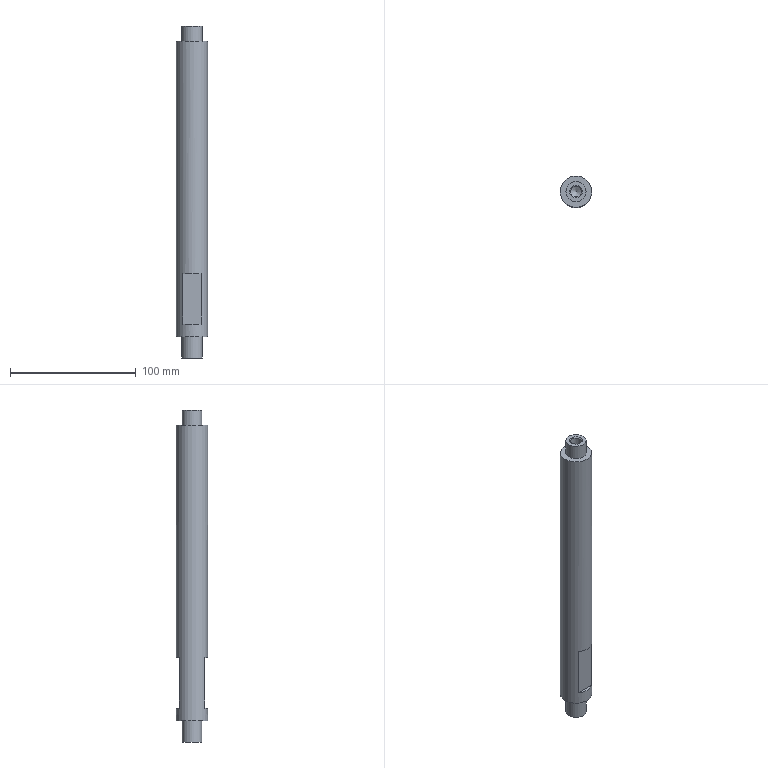Part | STEP file | YBQDJ-QD-PD-2 | 1 solid | 19 faces | box 25 x 25 x 264 mm | volume 116363 mm3 | plane 10 | cylinder 5 | cone 4 | commonest cylinder face diameters 8.5 x2 16 x2 25 x1
STEP:
#1=CARTESIAN_POINT('',(0.,0.,0.));
#2=DIRECTION('',(0.,0.,1.));
#3=DIRECTION('',(1.,0.,0.));
#4=AXIS2_PLACEMENT_3D('',#1,#2,#3);
#5=CARTESIAN_POINT('',(-327.5,-310.,260.));
#6=VERTEX_POINT('',#5);
#7=CARTESIAN_POINT('',(-340.,-310.,260.));
#8=DIRECTION('',(0.,0.,1.));
#9=DIRECTION('',(1.,0.,0.));
#10=AXIS2_PLACEMENT_3D('',#7,#8,#9);
#11=CIRCLE('',#10,12.5);
#12=CARTESIAN_POINT('',(-340.,-310.,270.));
#13=DIRECTION('',(0.,0.,-1.));
#14=DIRECTION('',(-1.,0.,0.));
#15=AXIS2_PLACEMENT_3D('',#12,#13,#14);
#16=CYLINDRICAL_SURFACE('',#15,12.5);
#17=CARTESIAN_POINT('',(9.425,10.));
#18=DIRECTION('',(-1.,0.));
#19=VECTOR('',#18,1.);
#20=LINE('',#17,#19);
#21=(GEOMETRIC_REPRESENTATION_CONTEXT(2)PARAMETRIC_REPRESENTATION_CONTEXT()REPRESENTATION_CONTEXT('',''));
#22=DEFINITIONAL_REPRESENTATION('',(#20),#21);
#23=PCURVE('',#16,#22);
#24=CARTESIAN_POINT('',(-340.,-310.,260.));
#25=DIRECTION('',(0.,0.,1.));
#26=DIRECTION('',(1.,0.,0.));
#27=AXIS2_PLACEMENT_3D('',#24,#25,#26);
#28=PLANE('',#27);
#29=CARTESIAN_POINT('',(0.,0.));
#30=DIRECTION('',(1.,0.));
#31=AXIS2_PLACEMENT_2D('',#29,#30);
#32=CIRCLE('',#31,12.5);
#33=(GEOMETRIC_REPRESENTATION_CONTEXT(2)PARAMETRIC_REPRESENTATION_CONTEXT()REPRESENTATION_CONTEXT('',''));
#34=DEFINITIONAL_REPRESENTATION('',(#32),#33);
#35=PCURVE('',#28,#34);
#36=SURFACE_CURVE('',#11,(#23,#35),.PCURVE_S1.);
#37=EDGE_CURVE('',#6,#6,#36,.T.);
#38=ORIENTED_EDGE('',*,*,#37,.F.);
#39=CARTESIAN_POINT('',(-327.5,-310.,25.));
#40=VERTEX_POINT('',#39);
#41=CARTESIAN_POINT('',(-327.5,-310.,260.));
#42=CARTESIAN_POINT('',(-327.5,-310.,25.));
#43=B_SPLINE_CURVE_WITH_KNOTS('',1,(#41,#42),.UNSPECIFIED.,.F.,.F.,(2,2),(10.,245.),.PIECEWISE_BEZIER_KNOTS.);
#44=CARTESIAN_POINT('',(9.425,0.));
#45=DIRECTION('',(0.,1.));
#46=VECTOR('',#45,1.);
#47=LINE('',#44,#46);
#48=(GEOMETRIC_REPRESENTATION_CONTEXT(2)PARAMETRIC_REPRESENTATION_CONTEXT()REPRESENTATION_CONTEXT('',''));
#49=DEFINITIONAL_REPRESENTATION('',(#47),#48);
#50=PCURVE('',#16,#49);
#51=CARTESIAN_POINT('',(3.142,0.));
#52=DIRECTION('',(0.,1.));
#53=VECTOR('',#52,1.);
#54=LINE('',#51,#53);
#55=(GEOMETRIC_REPRESENTATION_CONTEXT(2)PARAMETRIC_REPRESENTATION_CONTEXT()REPRESENTATION_CONTEXT('',''));
#56=DEFINITIONAL_REPRESENTATION('',(#54),#55);
#57=PCURVE('',#16,#56);
#58=SEAM_CURVE('',#43,(#50,#57),.PCURVE_S1.);
#59=EDGE_CURVE('',#6,#40,#58,.T.);
#60=ORIENTED_EDGE('',*,*,#59,.T.);
#61=CARTESIAN_POINT('',(-340.,-310.,25.));
#62=DIRECTION('',(0.,0.,1.));
#63=DIRECTION('',(1.,0.,0.));
#64=AXIS2_PLACEMENT_3D('',#61,#62,#63);
#65=CIRCLE('',#64,12.5);
#66=CARTESIAN_POINT('',(9.425,245.));
#67=DIRECTION('',(-1.,0.));
#68=VECTOR('',#67,1.);
#69=LINE('',#66,#68);
#70=(GEOMETRIC_REPRESENTATION_CONTEXT(2)PARAMETRIC_REPRESENTATION_CONTEXT()REPRESENTATION_CONTEXT('',''));
#71=DEFINITIONAL_REPRESENTATION('',(#69),#70);
#72=PCURVE('',#16,#71);
#73=CARTESIAN_POINT('',(92.5,10.,25.));
#74=DIRECTION('',(0.,0.,1.));
#75=DIRECTION('',(1.,0.,0.));
#76=AXIS2_PLACEMENT_3D('',#73,#74,#75);
#77=PLANE('',#76);
#78=CARTESIAN_POINT('',(-432.5,-320.));
#79=DIRECTION('',(1.,0.));
#80=AXIS2_PLACEMENT_2D('',#78,#79);
#81=CIRCLE('',#80,12.5);
#82=(GEOMETRIC_REPRESENTATION_CONTEXT(2)PARAMETRIC_REPRESENTATION_CONTEXT()REPRESENTATION_CONTEXT('',''));
#83=DEFINITIONAL_REPRESENTATION('',(#81),#82);
#84=PCURVE('',#77,#83);
#85=SURFACE_CURVE('',#65,(#72,#84),.PCURVE_S1.);
#86=EDGE_CURVE('',#40,#40,#85,.T.);
#87=ORIENTED_EDGE('',*,*,#86,.T.);
#88=ORIENTED_EDGE('',*,*,#59,.F.);
#89=EDGE_LOOP('',(#38,#60,#87,#88));
#90=FACE_BOUND('',#89,.T.);
#91=CARTESIAN_POINT('',(-347.5,-300.,75.));
#92=VERTEX_POINT('',#91);
#93=CARTESIAN_POINT('',(-332.5,-300.,75.));
#94=VERTEX_POINT('',#93);
#95=CARTESIAN_POINT('',(-340.,-310.,75.));
#96=DIRECTION('',(0.,0.,-1.));
#97=DIRECTION('',(0.,1.,0.));
#98=AXIS2_PLACEMENT_3D('',#95,#96,#97);
#99=CIRCLE('',#98,12.5);
#100=CARTESIAN_POINT('',(1.571,195.));
#101=DIRECTION('',(1.,0.));
#102=VECTOR('',#101,1.);
#103=LINE('',#100,#102);
#104=(GEOMETRIC_REPRESENTATION_CONTEXT(2)PARAMETRIC_REPRESENTATION_CONTEXT()REPRESENTATION_CONTEXT('',''));
#105=DEFINITIONAL_REPRESENTATION('',(#103),#104);
#106=PCURVE('',#16,#105);
#107=CARTESIAN_POINT('',(-382.,-300.,75.));
#108=DIRECTION('',(0.,0.,-1.));
#109=DIRECTION('',(0.,1.,0.));
#110=AXIS2_PLACEMENT_3D('',#107,#108,#109);
#111=PLANE('',#110);
#112=CARTESIAN_POINT('',(-10.,42.));
#113=DIRECTION('',(1.,0.));
#114=AXIS2_PLACEMENT_2D('',#112,#113);
#115=CIRCLE('',#114,12.5);
#116=(GEOMETRIC_REPRESENTATION_CONTEXT(2)PARAMETRIC_REPRESENTATION_CONTEXT()REPRESENTATION_CONTEXT('',''));
#117=DEFINITIONAL_REPRESENTATION('',(#115),#116);
#118=PCURVE('',#111,#117);
#119=SURFACE_CURVE('',#99,(#106,#118),.PCURVE_S1.);
#120=EDGE_CURVE('',#92,#94,#119,.T.);
#121=ORIENTED_EDGE('',*,*,#120,.F.);
#122=CARTESIAN_POINT('',(-347.5,-300.,35.));
#123=VERTEX_POINT('',#122);
#124=CARTESIAN_POINT('',(-347.5,-300.,270.));
#125=DIRECTION('',(0.,0.,1.));
#126=VECTOR('',#125,1.);
#127=LINE('',#124,#126);
#128=CARTESIAN_POINT('',(7.21,0.));
#129=DIRECTION('',(0.,-1.));
#130=VECTOR('',#129,1.);
#131=LINE('',#128,#130);
#132=(GEOMETRIC_REPRESENTATION_CONTEXT(2)PARAMETRIC_REPRESENTATION_CONTEXT()REPRESENTATION_CONTEXT('',''));
#133=DEFINITIONAL_REPRESENTATION('',(#131),#132);
#134=PCURVE('',#16,#133);
#135=CARTESIAN_POINT('',(-382.,-300.,35.));
#136=DIRECTION('',(0.,1.,0.));
#137=DIRECTION('',(0.,0.,1.));
#138=AXIS2_PLACEMENT_3D('',#135,#136,#137);
#139=PLANE('',#138);
#140=CARTESIAN_POINT('',(235.,34.5));
#141=DIRECTION('',(1.,0.));
#142=VECTOR('',#141,1.);
#143=LINE('',#140,#142);
#144=(GEOMETRIC_REPRESENTATION_CONTEXT(2)PARAMETRIC_REPRESENTATION_CONTEXT()REPRESENTATION_CONTEXT('',''));
#145=DEFINITIONAL_REPRESENTATION('',(#143),#144);
#146=PCURVE('',#139,#145);
#147=SURFACE_CURVE('',#127,(#134,#146),.PCURVE_S1.);
#148=EDGE_CURVE('',#123,#92,#147,.T.);
#149=ORIENTED_EDGE('',*,*,#148,.F.);
#150=CARTESIAN_POINT('',(-332.5,-300.,35.));
#151=VERTEX_POINT('',#150);
#152=CARTESIAN_POINT('',(-340.,-310.,35.));
#153=DIRECTION('',(0.,0.,1.));
#154=DIRECTION('',(0.,-1.,0.));
#155=AXIS2_PLACEMENT_3D('',#152,#153,#154);
#156=CIRCLE('',#155,12.5);
#157=CARTESIAN_POINT('',(10.996,235.));
#158=DIRECTION('',(-1.,0.));
#159=VECTOR('',#158,1.);
#160=LINE('',#157,#159);
#161=(GEOMETRIC_REPRESENTATION_CONTEXT(2)PARAMETRIC_REPRESENTATION_CONTEXT()REPRESENTATION_CONTEXT('',''));
#162=DEFINITIONAL_REPRESENTATION('',(#160),#161);
#163=PCURVE('',#16,#162);
#164=CARTESIAN_POINT('',(-382.,-281.,35.));
#165=DIRECTION('',(0.,0.,1.));
#166=DIRECTION('',(0.,-1.,0.));
#167=AXIS2_PLACEMENT_3D('',#164,#165,#166);
#168=PLANE('',#167);
#169=CARTESIAN_POINT('',(29.,42.));
#170=DIRECTION('',(1.,0.));
#171=AXIS2_PLACEMENT_2D('',#169,#170);
#172=CIRCLE('',#171,12.5);
#173=(GEOMETRIC_REPRESENTATION_CONTEXT(2)PARAMETRIC_REPRESENTATION_CONTEXT()REPRESENTATION_CONTEXT('',''));
#174=DEFINITIONAL_REPRESENTATION('',(#172),#173);
#175=PCURVE('',#168,#174);
#176=SURFACE_CURVE('',#156,(#163,#175),.PCURVE_S1.);
#177=EDGE_CURVE('',#151,#123,#176,.T.);
#178=ORIENTED_EDGE('',*,*,#177,.F.);
#179=CARTESIAN_POINT('',(-332.5,-300.,270.));
#180=DIRECTION('',(0.,0.,-1.));
#181=VECTOR('',#180,1.);
#182=LINE('',#179,#181);
#183=CARTESIAN_POINT('',(8.497,0.));
#184=DIRECTION('',(0.,1.));
#185=VECTOR('',#184,1.);
#186=LINE('',#183,#185);
#187=(GEOMETRIC_REPRESENTATION_CONTEXT(2)PARAMETRIC_REPRESENTATION_CONTEXT()REPRESENTATION_CONTEXT('',''));
#188=DEFINITIONAL_REPRESENTATION('',(#186),#187);
#189=PCURVE('',#16,#188);
#190=CARTESIAN_POINT('',(235.,49.5));
#191=DIRECTION('',(-1.,0.));
#192=VECTOR('',#191,1.);
#193=LINE('',#190,#192);
#194=(GEOMETRIC_REPRESENTATION_CONTEXT(2)PARAMETRIC_REPRESENTATION_CONTEXT()REPRESENTATION_CONTEXT('',''));
#195=DEFINITIONAL_REPRESENTATION('',(#193),#194);
#196=PCURVE('',#139,#195);
#197=SURFACE_CURVE('',#182,(#189,#196),.PCURVE_S1.);
#198=EDGE_CURVE('',#94,#151,#197,.T.);
#199=ORIENTED_EDGE('',*,*,#198,.F.);
#200=EDGE_LOOP('',(#121,#149,#178,#199));
#201=FACE_BOUND('',#200,.T.);
#202=CARTESIAN_POINT('',(-332.5,-320.,75.));
#203=VERTEX_POINT('',#202);
#204=CARTESIAN_POINT('',(-347.5,-320.,75.));
#205=VERTEX_POINT('',#204);
#206=CARTESIAN_POINT('',(-340.,-310.,75.));
#207=DIRECTION('',(0.,0.,-1.));
#208=DIRECTION('',(0.,1.,0.));
#209=AXIS2_PLACEMENT_3D('',#206,#207,#208);
#210=CIRCLE('',#209,12.5);
#211=CARTESIAN_POINT('',(1.571,195.));
#212=DIRECTION('',(1.,0.));
#213=VECTOR('',#212,1.);
#214=LINE('',#211,#213);
#215=(GEOMETRIC_REPRESENTATION_CONTEXT(2)PARAMETRIC_REPRESENTATION_CONTEXT()REPRESENTATION_CONTEXT('',''));
#216=DEFINITIONAL_REPRESENTATION('',(#214),#215);
#217=PCURVE('',#16,#216);
#218=CARTESIAN_POINT('',(-382.,-339.,75.));
#219=DIRECTION('',(0.,0.,-1.));
#220=DIRECTION('',(0.,1.,0.));
#221=AXIS2_PLACEMENT_3D('',#218,#219,#220);
#222=PLANE('',#221);
#223=CARTESIAN_POINT('',(29.,42.));
#224=DIRECTION('',(1.,0.));
#225=AXIS2_PLACEMENT_2D('',#223,#224);
#226=CIRCLE('',#225,12.5);
#227=(GEOMETRIC_REPRESENTATION_CONTEXT(2)PARAMETRIC_REPRESENTATION_CONTEXT()REPRESENTATION_CONTEXT('',''));
#228=DEFINITIONAL_REPRESENTATION('',(#226),#227);
#229=PCURVE('',#222,#228);
#230=SURFACE_CURVE('',#210,(#217,#229),.PCURVE_S1.);
#231=EDGE_CURVE('',#203,#205,#230,.T.);
#232=ORIENTED_EDGE('',*,*,#231,.F.);
#233=CARTESIAN_POINT('',(-332.5,-320.,35.));
#234=VERTEX_POINT('',#233);
#235=CARTESIAN_POINT('',(-332.5,-320.,270.));
#236=DIRECTION('',(0.,0.,1.));
#237=VECTOR('',#236,1.);
#238=LINE('',#235,#237);
#239=CARTESIAN_POINT('',(4.069,0.));
#240=DIRECTION('',(0.,-1.));
#241=VECTOR('',#240,1.);
#242=LINE('',#239,#241);
#243=(GEOMETRIC_REPRESENTATION_CONTEXT(2)PARAMETRIC_REPRESENTATION_CONTEXT()REPRESENTATION_CONTEXT('',''));
#244=DEFINITIONAL_REPRESENTATION('',(#242),#243);
#245=PCURVE('',#16,#244);
#246=CARTESIAN_POINT('',(-382.,-320.,65.));
#247=DIRECTION('',(0.,-1.,0.));
#248=DIRECTION('',(0.,0.,-1.));
#249=AXIS2_PLACEMENT_3D('',#246,#247,#248);
#250=PLANE('',#249);
#251=CARTESIAN_POINT('',(-205.,49.5));
#252=DIRECTION('',(-1.,0.));
#253=VECTOR('',#252,1.);
#254=LINE('',#251,#253);
#255=(GEOMETRIC_REPRESENTATION_CONTEXT(2)PARAMETRIC_REPRESENTATION_CONTEXT()REPRESENTATION_CONTEXT('',''));
#256=DEFINITIONAL_REPRESENTATION('',(#254),#255);
#257=PCURVE('',#250,#256);
#258=SURFACE_CURVE('',#238,(#245,#257),.PCURVE_S1.);
#259=EDGE_CURVE('',#234,#203,#258,.T.);
#260=ORIENTED_EDGE('',*,*,#259,.F.);
#261=CARTESIAN_POINT('',(-347.5,-320.,35.));
#262=VERTEX_POINT('',#261);
#263=CARTESIAN_POINT('',(-340.,-310.,35.));
#264=DIRECTION('',(0.,0.,1.));
#265=DIRECTION('',(0.,-1.,0.));
#266=AXIS2_PLACEMENT_3D('',#263,#264,#265);
#267=CIRCLE('',#266,12.5);
#268=CARTESIAN_POINT('',(10.996,235.));
#269=DIRECTION('',(-1.,0.));
#270=VECTOR('',#269,1.);
#271=LINE('',#268,#270);
#272=(GEOMETRIC_REPRESENTATION_CONTEXT(2)PARAMETRIC_REPRESENTATION_CONTEXT()REPRESENTATION_CONTEXT('',''));
#273=DEFINITIONAL_REPRESENTATION('',(#271),#272);
#274=PCURVE('',#16,#273);
#275=CARTESIAN_POINT('',(-382.,-320.,35.));
#276=DIRECTION('',(0.,0.,1.));
#277=DIRECTION('',(0.,-1.,0.));
#278=AXIS2_PLACEMENT_3D('',#275,#276,#277);
#279=PLANE('',#278);
#280=CARTESIAN_POINT('',(-10.,42.));
#281=DIRECTION('',(1.,0.));
#282=AXIS2_PLACEMENT_2D('',#280,#281);
#283=CIRCLE('',#282,12.5);
#284=(GEOMETRIC_REPRESENTATION_CONTEXT(2)PARAMETRIC_REPRESENTATION_CONTEXT()REPRESENTATION_CONTEXT('',''));
#285=DEFINITIONAL_REPRESENTATION('',(#283),#284);
#286=PCURVE('',#279,#285);
#287=SURFACE_CURVE('',#267,(#274,#286),.PCURVE_S1.);
#288=EDGE_CURVE('',#262,#234,#287,.T.);
#289=ORIENTED_EDGE('',*,*,#288,.F.);
#290=CARTESIAN_POINT('',(-347.5,-320.,270.));
#291=DIRECTION('',(0.,0.,-1.));
#292=VECTOR('',#291,1.);
#293=LINE('',#290,#292);
#294=CARTESIAN_POINT('',(5.356,0.));
#295=DIRECTION('',(0.,1.));
#296=VECTOR('',#295,1.);
#297=LINE('',#294,#296);
#298=(GEOMETRIC_REPRESENTATION_CONTEXT(2)PARAMETRIC_REPRESENTATION_CONTEXT()REPRESENTATION_CONTEXT('',''));
#299=DEFINITIONAL_REPRESENTATION('',(#297),#298);
#300=PCURVE('',#16,#299);
#301=CARTESIAN_POINT('',(-205.,34.5));
#302=DIRECTION('',(1.,0.));
#303=VECTOR('',#302,1.);
#304=LINE('',#301,#303);
#305=(GEOMETRIC_REPRESENTATION_CONTEXT(2)PARAMETRIC_REPRESENTATION_CONTEXT()REPRESENTATION_CONTEXT('',''));
#306=DEFINITIONAL_REPRESENTATION('',(#304),#305);
#307=PCURVE('',#250,#306);
#308=SURFACE_CURVE('',#293,(#300,#307),.PCURVE_S1.);
#309=EDGE_CURVE('',#205,#262,#308,.T.);
#310=ORIENTED_EDGE('',*,*,#309,.F.);
#311=EDGE_LOOP('',(#232,#260,#289,#310));
#312=FACE_BOUND('',#311,.T.);
#313=ADVANCED_FACE('',(#90,#201,#312),#16,.T.);
#314=CARTESIAN_POINT('',(-332.,-310.,260.));
#315=VERTEX_POINT('',#314);
#316=CARTESIAN_POINT('',(-340.,-310.,260.));
#317=DIRECTION('',(0.,0.,1.));
#318=DIRECTION('',(1.,0.,0.));
#319=AXIS2_PLACEMENT_3D('',#316,#317,#318);
#320=CIRCLE('',#319,8.);
#321=CARTESIAN_POINT('',(0.,0.));
#322=DIRECTION('',(1.,0.));
#323=AXIS2_PLACEMENT_2D('',#321,#322);
#324=CIRCLE('',#323,8.);
#325=(GEOMETRIC_REPRESENTATION_CONTEXT(2)PARAMETRIC_REPRESENTATION_CONTEXT()REPRESENTATION_CONTEXT('',''));
#326=DEFINITIONAL_REPRESENTATION('',(#324),#325);
#327=PCURVE('',#28,#326);
#328=CARTESIAN_POINT('',(-340.,-310.,275.));
#329=DIRECTION('',(0.,0.,-1.));
#330=DIRECTION('',(-1.,0.,0.));
#331=AXIS2_PLACEMENT_3D('',#328,#329,#330);
#332=CYLINDRICAL_SURFACE('',#331,8.);
#333=CARTESIAN_POINT('',(9.425,15.));
#334=DIRECTION('',(-1.,0.));
#335=VECTOR('',#334,1.);
#336=LINE('',#333,#335);
#337=(GEOMETRIC_REPRESENTATION_CONTEXT(2)PARAMETRIC_REPRESENTATION_CONTEXT()REPRESENTATION_CONTEXT('',''));
#338=DEFINITIONAL_REPRESENTATION('',(#336),#337);
#339=PCURVE('',#332,#338);
#340=SURFACE_CURVE('',#320,(#327,#339),.PCURVE_S1.);
#341=EDGE_CURVE('',#315,#315,#340,.T.);
#342=ORIENTED_EDGE('',*,*,#341,.F.);
#343=EDGE_LOOP('',(#342));
#344=FACE_BOUND('',#343,.T.);
#345=ORIENTED_EDGE('',*,*,#37,.T.);
#346=EDGE_LOOP('',(#345));
#347=FACE_BOUND('',#346,.T.);
#348=ADVANCED_FACE('',(#344,#347),#28,.T.);
#349=CARTESIAN_POINT('',(-332.,-310.,25.));
#350=VERTEX_POINT('',#349);
#351=CARTESIAN_POINT('',(-340.,-310.,25.));
#352=DIRECTION('',(0.,0.,-1.));
#353=DIRECTION('',(1.,0.,0.));
#354=AXIS2_PLACEMENT_3D('',#351,#352,#353);
#355=CIRCLE('',#354,8.);
#356=CARTESIAN_POINT('',(-424.5,-320.));
#357=CARTESIAN_POINT('',(-424.5,-333.856));
#358=CARTESIAN_POINT('',(-436.5,-326.928));
#359=CARTESIAN_POINT('',(-448.5,-320.));
#360=CARTESIAN_POINT('',(-436.5,-313.072));
#361=CARTESIAN_POINT('',(-424.5,-306.144));
#362=CARTESIAN_POINT('',(-424.5,-320.));
#363=(BOUNDED_CURVE()B_SPLINE_CURVE(2,(#356,#357,#358,#359,#360,#361,#362),.UNSPECIFIED.,.T.,.F.)B_SPLINE_CURVE_WITH_KNOTS((1,2,2,2,2,1),(-2.094,0.,2.094,4.189,6.283,8.378),.UNSPECIFIED.)CURVE()GEOMETRIC_REPRESENTATION_ITEM()RATIONAL_B_SPLINE_CURVE((1.,0.5,1.,0.5,1.,0.5,1.))REPRESENTATION_ITEM(''));
#364=(GEOMETRIC_REPRESENTATION_CONTEXT(2)PARAMETRIC_REPRESENTATION_CONTEXT()REPRESENTATION_CONTEXT('',''));
#365=DEFINITIONAL_REPRESENTATION('',(#363),#364);
#366=PCURVE('',#77,#365);
#367=CARTESIAN_POINT('',(-340.,-310.,8.));
#368=DIRECTION('',(0.,0.,1.));
#369=DIRECTION('',(1.,0.,0.));
#370=AXIS2_PLACEMENT_3D('',#367,#368,#369);
#371=CYLINDRICAL_SURFACE('',#370,8.);
#372=CARTESIAN_POINT('',(6.283,17.));
#373=DIRECTION('',(-1.,0.));
#374=VECTOR('',#373,1.);
#375=LINE('',#372,#374);
#376=(GEOMETRIC_REPRESENTATION_CONTEXT(2)PARAMETRIC_REPRESENTATION_CONTEXT()REPRESENTATION_CONTEXT('',''));
#377=DEFINITIONAL_REPRESENTATION('',(#375),#376);
#378=PCURVE('',#371,#377);
#379=SURFACE_CURVE('',#355,(#366,#378),.PCURVE_S1.);
#380=EDGE_CURVE('',#350,#350,#379,.T.);
#381=ORIENTED_EDGE('',*,*,#380,.F.);
#382=EDGE_LOOP('',(#381));
#383=FACE_BOUND('',#382,.T.);
#384=ORIENTED_EDGE('',*,*,#86,.F.);
#385=EDGE_LOOP('',(#384));
#386=FACE_BOUND('',#385,.T.);
#387=ADVANCED_FACE('',(#383,#386),#77,.F.);
#388=CARTESIAN_POINT('',(-332.,-310.,272.));
#389=VERTEX_POINT('',#388);
#390=CARTESIAN_POINT('',(-340.,-310.,272.));
#391=DIRECTION('',(0.,0.,1.));
#392=DIRECTION('',(1.,0.,0.));
#393=AXIS2_PLACEMENT_3D('',#390,#391,#392);
#394=CIRCLE('',#393,8.);
#395=CARTESIAN_POINT('',(9.425,3.));
#396=DIRECTION('',(-1.,0.));
#397=VECTOR('',#396,1.);
#398=LINE('',#395,#397);
#399=(GEOMETRIC_REPRESENTATION_CONTEXT(2)PARAMETRIC_REPRESENTATION_CONTEXT()REPRESENTATION_CONTEXT('',''));
#400=DEFINITIONAL_REPRESENTATION('',(#398),#399);
#401=PCURVE('',#332,#400);
#402=CARTESIAN_POINT('',(-340.,-310.,272.));
#403=DIRECTION('',(0.,0.,1.));
#404=DIRECTION('',(1.,0.,0.));
#405=AXIS2_PLACEMENT_3D('',#402,#403,#404);
#406=PLANE('',#405);
#407=CARTESIAN_POINT('',(0.,0.));
#408=DIRECTION('',(1.,0.));
#409=AXIS2_PLACEMENT_2D('',#407,#408);
#410=CIRCLE('',#409,8.);
#411=(GEOMETRIC_REPRESENTATION_CONTEXT(2)PARAMETRIC_REPRESENTATION_CONTEXT()REPRESENTATION_CONTEXT('',''));
#412=DEFINITIONAL_REPRESENTATION('',(#410),#411);
#413=PCURVE('',#406,#412);
#414=SURFACE_CURVE('',#394,(#401,#413),.PCURVE_S1.);
#415=EDGE_CURVE('',#389,#389,#414,.T.);
#416=ORIENTED_EDGE('',*,*,#415,.F.);
#417=CARTESIAN_POINT('',(-332.,-310.,272.));
#418=CARTESIAN_POINT('',(-332.,-310.,260.));
#419=B_SPLINE_CURVE_WITH_KNOTS('',1,(#417,#418),.UNSPECIFIED.,.F.,.F.,(2,2),(3.,15.),.PIECEWISE_BEZIER_KNOTS.);
#420=CARTESIAN_POINT('',(9.425,0.));
#421=DIRECTION('',(0.,1.));
#422=VECTOR('',#421,1.);
#423=LINE('',#420,#422);
#424=(GEOMETRIC_REPRESENTATION_CONTEXT(2)PARAMETRIC_REPRESENTATION_CONTEXT()REPRESENTATION_CONTEXT('',''));
#425=DEFINITIONAL_REPRESENTATION('',(#423),#424);
#426=PCURVE('',#332,#425);
#427=CARTESIAN_POINT('',(3.142,0.));
#428=DIRECTION('',(0.,1.));
#429=VECTOR('',#428,1.);
#430=LINE('',#427,#429);
#431=(GEOMETRIC_REPRESENTATION_CONTEXT(2)PARAMETRIC_REPRESENTATION_CONTEXT()REPRESENTATION_CONTEXT('',''));
#432=DEFINITIONAL_REPRESENTATION('',(#430),#431);
#433=PCURVE('',#332,#432);
#434=SEAM_CURVE('',#419,(#426,#433),.PCURVE_S1.);
#435=EDGE_CURVE('',#389,#315,#434,.T.);
#436=ORIENTED_EDGE('',*,*,#435,.T.);
#437=ORIENTED_EDGE('',*,*,#341,.T.);
#438=ORIENTED_EDGE('',*,*,#435,.F.);
#439=EDGE_LOOP('',(#416,#436,#437,#438));
#440=FACE_BOUND('',#439,.T.);
#441=ADVANCED_FACE('',(#440),#332,.T.);
#442=CARTESIAN_POINT('',(-335.,-310.,272.));
#443=VERTEX_POINT('',#442);
#444=CARTESIAN_POINT('',(-340.,-310.,272.));
#445=DIRECTION('',(0.,0.,-1.));
#446=DIRECTION('',(1.,0.,0.));
#447=AXIS2_PLACEMENT_3D('',#444,#445,#446);
#448=CIRCLE('',#447,5.);
#449=CARTESIAN_POINT('',(5.,0.));
#450=CARTESIAN_POINT('',(5.,-8.66));
#451=CARTESIAN_POINT('',(-2.5,-4.33));
#452=CARTESIAN_POINT('',(-10.,0.));
#453=CARTESIAN_POINT('',(-2.5,4.33));
#454=CARTESIAN_POINT('',(5.,8.66));
#455=CARTESIAN_POINT('',(5.,0.));
#456=(BOUNDED_CURVE()B_SPLINE_CURVE(2,(#449,#450,#451,#452,#453,#454,#455),.UNSPECIFIED.,.T.,.F.)B_SPLINE_CURVE_WITH_KNOTS((1,2,2,2,2,1),(-2.094,0.,2.094,4.189,6.283,8.378),.UNSPECIFIED.)CURVE()GEOMETRIC_REPRESENTATION_ITEM()RATIONAL_B_SPLINE_CURVE((1.,0.5,1.,0.5,1.,0.5,1.))REPRESENTATION_ITEM(''));
#457=(GEOMETRIC_REPRESENTATION_CONTEXT(2)PARAMETRIC_REPRESENTATION_CONTEXT()REPRESENTATION_CONTEXT('',''));
#458=DEFINITIONAL_REPRESENTATION('',(#456),#457);
#459=PCURVE('',#406,#458);
#460=CARTESIAN_POINT('',(-340.,-310.,272.));
#461=DIRECTION('',(0.,0.,1.));
#462=DIRECTION('',(1.,0.,0.));
#463=AXIS2_PLACEMENT_3D('',#460,#461,#462);
#464=CONICAL_SURFACE('',#463,5.,0.7854);
#465=CARTESIAN_POINT('',(6.283,0.));
#466=DIRECTION('',(-1.,0.));
#467=VECTOR('',#466,1.);
#468=LINE('',#465,#467);
#469=(GEOMETRIC_REPRESENTATION_CONTEXT(2)PARAMETRIC_REPRESENTATION_CONTEXT()REPRESENTATION_CONTEXT('',''));
#470=DEFINITIONAL_REPRESENTATION('',(#468),#469);
#471=PCURVE('',#464,#470);
#472=SURFACE_CURVE('',#448,(#459,#471),.PCURVE_S1.);
#473=EDGE_CURVE('',#443,#443,#472,.T.);
#474=ORIENTED_EDGE('',*,*,#473,.T.);
#475=EDGE_LOOP('',(#474));
#476=FACE_BOUND('',#475,.T.);
#477=ORIENTED_EDGE('',*,*,#415,.T.);
#478=EDGE_LOOP('',(#477));
#479=FACE_BOUND('',#478,.T.);
#480=ADVANCED_FACE('',(#476,#479),#406,.T.);
#481=CARTESIAN_POINT('',(-335.75,-310.,250.));
#482=VERTEX_POINT('',#481);
#483=CARTESIAN_POINT('',(-344.25,-310.,250.));
#484=VERTEX_POINT('',#483);
#485=CARTESIAN_POINT('',(-340.,-310.,250.));
#486=DIRECTION('',(0.,0.,1.));
#487=DIRECTION('',(-1.,0.,0.));
#488=AXIS2_PLACEMENT_3D('',#485,#486,#487);
#489=CIRCLE('',#488,4.25);
#490=CARTESIAN_POINT('',(-340.,-310.,250.));
#491=DIRECTION('',(0.,0.,1.));
#492=DIRECTION('',(1.,0.,0.));
#493=AXIS2_PLACEMENT_3D('',#490,#491,#492);
#494=CONICAL_SURFACE('',#493,4.25,1.03);
#495=CARTESIAN_POINT('',(-3.142,0.));
#496=DIRECTION('',(1.,0.));
#497=VECTOR('',#496,1.);
#498=LINE('',#495,#497);
#499=(GEOMETRIC_REPRESENTATION_CONTEXT(2)PARAMETRIC_REPRESENTATION_CONTEXT()REPRESENTATION_CONTEXT('',''));
#500=DEFINITIONAL_REPRESENTATION('',(#498),#499);
#501=PCURVE('',#494,#500);
#502=CARTESIAN_POINT('',(-340.,-310.,275.));
#503=DIRECTION('',(0.,0.,-1.));
#504=DIRECTION('',(-1.,0.,0.));
#505=AXIS2_PLACEMENT_3D('',#502,#503,#504);
#506=CYLINDRICAL_SURFACE('',#505,4.25);
#507=CARTESIAN_POINT('',(12.566,25.));
#508=DIRECTION('',(-1.,0.));
#509=VECTOR('',#508,1.);
#510=LINE('',#507,#509);
#511=(GEOMETRIC_REPRESENTATION_CONTEXT(2)PARAMETRIC_REPRESENTATION_CONTEXT()REPRESENTATION_CONTEXT('',''));
#512=DEFINITIONAL_REPRESENTATION('',(#510),#511);
#513=PCURVE('',#506,#512);
#514=SURFACE_CURVE('',#489,(#501,#513),.PCURVE_S1.);
#515=EDGE_CURVE('',#482,#484,#514,.T.);
#516=ORIENTED_EDGE('',*,*,#515,.F.);
#517=CARTESIAN_POINT('',(-340.,-310.,247.446));
#518=VERTEX_POINT('',#517);
#519=CARTESIAN_POINT('',(-340.,-310.,247.446));
#520=CARTESIAN_POINT('',(-335.75,-310.,250.));
#521=B_SPLINE_CURVE_WITH_KNOTS('',1,(#519,#520),.UNSPECIFIED.,.F.,.F.,(2,2),(-4.958,0.),.PIECEWISE_BEZIER_KNOTS.);
#522=CARTESIAN_POINT('',(0.,0.));
#523=DIRECTION('',(0.,1.));
#524=VECTOR('',#523,1.);
#525=LINE('',#522,#524);
#526=(GEOMETRIC_REPRESENTATION_CONTEXT(2)PARAMETRIC_REPRESENTATION_CONTEXT()REPRESENTATION_CONTEXT('',''));
#527=DEFINITIONAL_REPRESENTATION('',(#525),#526);
#528=PCURVE('',#494,#527);
#529=CARTESIAN_POINT('',(6.283,0.));
#530=DIRECTION('',(0.,1.));
#531=VECTOR('',#530,1.);
#532=LINE('',#529,#531);
#533=(GEOMETRIC_REPRESENTATION_CONTEXT(2)PARAMETRIC_REPRESENTATION_CONTEXT()REPRESENTATION_CONTEXT('',''));
#534=DEFINITIONAL_REPRESENTATION('',(#532),#533);
#535=PCURVE('',#494,#534);
#536=SEAM_CURVE('',#521,(#528,#535),.PCURVE_S1.);
#537=EDGE_CURVE('',#518,#482,#536,.T.);
#538=ORIENTED_EDGE('',*,*,#537,.F.);
#539=ORIENTED_EDGE('',*,*,#537,.T.);
#540=CARTESIAN_POINT('',(-340.,-310.,250.));
#541=DIRECTION('',(0.,0.,1.));
#542=DIRECTION('',(-1.,0.,0.));
#543=AXIS2_PLACEMENT_3D('',#540,#541,#542);
#544=CIRCLE('',#543,4.25);
#545=CARTESIAN_POINT('',(3.142,0.));
#546=DIRECTION('',(1.,0.));
#547=VECTOR('',#546,1.);
#548=LINE('',#545,#547);
#549=(GEOMETRIC_REPRESENTATION_CONTEXT(2)PARAMETRIC_REPRESENTATION_CONTEXT()REPRESENTATION_CONTEXT('',''));
#550=DEFINITIONAL_REPRESENTATION('',(#548),#549);
#551=PCURVE('',#494,#550);
#552=CARTESIAN_POINT('',(6.283,25.));
#553=DIRECTION('',(-1.,0.));
#554=VECTOR('',#553,1.);
#555=LINE('',#552,#554);
#556=(GEOMETRIC_REPRESENTATION_CONTEXT(2)PARAMETRIC_REPRESENTATION_CONTEXT()REPRESENTATION_CONTEXT('',''));
#557=DEFINITIONAL_REPRESENTATION('',(#555),#556);
#558=PCURVE('',#506,#557);
#559=SURFACE_CURVE('',#544,(#551,#558),.PCURVE_S1.);
#560=EDGE_CURVE('',#484,#482,#559,.T.);
#561=ORIENTED_EDGE('',*,*,#560,.F.);
#562=EDGE_LOOP('',(#516,#538,#539,#561));
#563=FACE_BOUND('',#562,.F.);
#564=ADVANCED_FACE('',(#563),#494,.F.);
#565=CARTESIAN_POINT('',(-335.75,-310.,271.25));
#566=VERTEX_POINT('',#565);
#567=CARTESIAN_POINT('',(-340.,-310.,271.25));
#568=DIRECTION('',(0.,0.,1.));
#569=DIRECTION('',(1.,0.,0.));
#570=AXIS2_PLACEMENT_3D('',#567,#568,#569);
#571=CIRCLE('',#570,4.25);
#572=CARTESIAN_POINT('',(9.425,3.75));
#573=DIRECTION('',(-1.,0.));
#574=VECTOR('',#573,1.);
#575=LINE('',#572,#574);
#576=(GEOMETRIC_REPRESENTATION_CONTEXT(2)PARAMETRIC_REPRESENTATION_CONTEXT()REPRESENTATION_CONTEXT('',''));
#577=DEFINITIONAL_REPRESENTATION('',(#575),#576);
#578=PCURVE('',#506,#577);
#579=CARTESIAN_POINT('',(0.,-0.75));
#580=DIRECTION('',(1.,0.));
#581=VECTOR('',#580,1.);
#582=LINE('',#579,#581);
#583=(GEOMETRIC_REPRESENTATION_CONTEXT(2)PARAMETRIC_REPRESENTATION_CONTEXT()REPRESENTATION_CONTEXT('',''));
#584=DEFINITIONAL_REPRESENTATION('',(#582),#583);
#585=PCURVE('',#464,#584);
#586=SURFACE_CURVE('',#571,(#578,#585),.PCURVE_S1.);
#587=EDGE_CURVE('',#566,#566,#586,.T.);
#588=ORIENTED_EDGE('',*,*,#587,.F.);
#589=CARTESIAN_POINT('',(-335.75,-310.,271.25));
#590=CARTESIAN_POINT('',(-335.75,-310.,250.));
#591=B_SPLINE_CURVE_WITH_KNOTS('',1,(#589,#590),.UNSPECIFIED.,.F.,.F.,(2,2),(3.75,25.),.PIECEWISE_BEZIER_KNOTS.);
#592=CARTESIAN_POINT('',(9.425,0.));
#593=DIRECTION('',(0.,1.));
#594=VECTOR('',#593,1.);
#595=LINE('',#592,#594);
#596=(GEOMETRIC_REPRESENTATION_CONTEXT(2)PARAMETRIC_REPRESENTATION_CONTEXT()REPRESENTATION_CONTEXT('',''));
#597=DEFINITIONAL_REPRESENTATION('',(#595),#596);
#598=PCURVE('',#506,#597);
#599=CARTESIAN_POINT('',(3.142,0.));
#600=DIRECTION('',(0.,1.));
#601=VECTOR('',#600,1.);
#602=LINE('',#599,#601);
#603=(GEOMETRIC_REPRESENTATION_CONTEXT(2)PARAMETRIC_REPRESENTATION_CONTEXT()REPRESENTATION_CONTEXT('',''));
#604=DEFINITIONAL_REPRESENTATION('',(#602),#603);
#605=PCURVE('',#506,#604);
#606=SEAM_CURVE('',#591,(#598,#605),.PCURVE_S1.);
#607=EDGE_CURVE('',#566,#482,#606,.T.);
#608=ORIENTED_EDGE('',*,*,#607,.T.);
#609=ORIENTED_EDGE('',*,*,#515,.T.);
#610=ORIENTED_EDGE('',*,*,#560,.T.);
#611=ORIENTED_EDGE('',*,*,#607,.F.);
#612=EDGE_LOOP('',(#588,#608,#609,#610,#611));
#613=FACE_BOUND('',#612,.F.);
#614=ADVANCED_FACE('',(#613),#506,.F.);
#615=ORIENTED_EDGE('',*,*,#587,.T.);
#616=CARTESIAN_POINT('',(-335.75,-310.,271.25));
#617=CARTESIAN_POINT('',(-335.,-310.,272.));
#618=B_SPLINE_CURVE_WITH_KNOTS('',1,(#616,#617),.UNSPECIFIED.,.F.,.F.,(2,2),(-1.061,0.),.PIECEWISE_BEZIER_KNOTS.);
#619=CARTESIAN_POINT('',(6.283,0.));
#620=DIRECTION('',(0.,1.));
#621=VECTOR('',#620,1.);
#622=LINE('',#619,#621);
#623=(GEOMETRIC_REPRESENTATION_CONTEXT(2)PARAMETRIC_REPRESENTATION_CONTEXT()REPRESENTATION_CONTEXT('',''));
#624=DEFINITIONAL_REPRESENTATION('',(#622),#623);
#625=PCURVE('',#464,#624);
#626=CARTESIAN_POINT('',(0.,0.));
#627=DIRECTION('',(0.,1.));
#628=VECTOR('',#627,1.);
#629=LINE('',#626,#628);
#630=(GEOMETRIC_REPRESENTATION_CONTEXT(2)PARAMETRIC_REPRESENTATION_CONTEXT()REPRESENTATION_CONTEXT('',''));
#631=DEFINITIONAL_REPRESENTATION('',(#629),#630);
#632=PCURVE('',#464,#631);
#633=SEAM_CURVE('',#618,(#625,#632),.PCURVE_S1.);
#634=EDGE_CURVE('',#566,#443,#633,.T.);
#635=ORIENTED_EDGE('',*,*,#634,.T.);
#636=ORIENTED_EDGE('',*,*,#473,.T.);
#637=ORIENTED_EDGE('',*,*,#634,.F.);
#638=EDGE_LOOP('',(#615,#635,#636,#637));
#639=FACE_BOUND('',#638,.F.);
#640=ADVANCED_FACE('',(#639),#464,.F.);
#641=CARTESIAN_POINT('',(-332.,-310.,8.));
#642=VERTEX_POINT('',#641);
#643=CARTESIAN_POINT('',(-348.,-310.,8.));
#644=VERTEX_POINT('',#643);
#645=CARTESIAN_POINT('',(-340.,-310.,8.));
#646=DIRECTION('',(0.,0.,-1.));
#647=DIRECTION('',(-1.,0.,0.));
#648=AXIS2_PLACEMENT_3D('',#645,#646,#647);
#649=CIRCLE('',#648,8.);
#650=CARTESIAN_POINT('',(9.425,0.));
#651=DIRECTION('',(-1.,0.));
#652=VECTOR('',#651,1.);
#653=LINE('',#650,#652);
#654=(GEOMETRIC_REPRESENTATION_CONTEXT(2)PARAMETRIC_REPRESENTATION_CONTEXT()REPRESENTATION_CONTEXT('',''));
#655=DEFINITIONAL_REPRESENTATION('',(#653),#654);
#656=PCURVE('',#371,#655);
#657=CARTESIAN_POINT('',(-340.,-310.,8.));
#658=DIRECTION('',(0.,0.,-1.));
#659=DIRECTION('',(-1.,0.,0.));
#660=AXIS2_PLACEMENT_3D('',#657,#658,#659);
#661=PLANE('',#660);
#662=CARTESIAN_POINT('',(0.,0.));
#663=DIRECTION('',(1.,0.));
#664=AXIS2_PLACEMENT_2D('',#662,#663);
#665=CIRCLE('',#664,8.);
#666=(GEOMETRIC_REPRESENTATION_CONTEXT(2)PARAMETRIC_REPRESENTATION_CONTEXT()REPRESENTATION_CONTEXT('',''));
#667=DEFINITIONAL_REPRESENTATION('',(#665),#666);
#668=PCURVE('',#661,#667);
#669=SURFACE_CURVE('',#649,(#656,#668),.PCURVE_S1.);
#670=EDGE_CURVE('',#642,#644,#669,.T.);
#671=ORIENTED_EDGE('',*,*,#670,.F.);
#672=CARTESIAN_POINT('',(-332.,-310.,8.));
#673=CARTESIAN_POINT('',(-332.,-310.,25.));
#674=B_SPLINE_CURVE_WITH_KNOTS('',1,(#672,#673),.UNSPECIFIED.,.F.,.F.,(2,2),(0.,17.),.PIECEWISE_BEZIER_KNOTS.);
#675=CARTESIAN_POINT('',(6.283,0.));
#676=DIRECTION('',(0.,1.));
#677=VECTOR('',#676,1.);
#678=LINE('',#675,#677);
#679=(GEOMETRIC_REPRESENTATION_CONTEXT(2)PARAMETRIC_REPRESENTATION_CONTEXT()REPRESENTATION_CONTEXT('',''));
#680=DEFINITIONAL_REPRESENTATION('',(#678),#679);
#681=PCURVE('',#371,#680);
#682=CARTESIAN_POINT('',(0.,0.));
#683=DIRECTION('',(0.,1.));
#684=VECTOR('',#683,1.);
#685=LINE('',#682,#684);
#686=(GEOMETRIC_REPRESENTATION_CONTEXT(2)PARAMETRIC_REPRESENTATION_CONTEXT()REPRESENTATION_CONTEXT('',''));
#687=DEFINITIONAL_REPRESENTATION('',(#685),#686);
#688=PCURVE('',#371,#687);
#689=SEAM_CURVE('',#674,(#681,#688),.PCURVE_S1.);
#690=EDGE_CURVE('',#642,#350,#689,.T.);
#691=ORIENTED_EDGE('',*,*,#690,.T.);
#692=ORIENTED_EDGE('',*,*,#380,.T.);
#693=ORIENTED_EDGE('',*,*,#690,.F.);
#694=CARTESIAN_POINT('',(-340.,-310.,8.));
#695=DIRECTION('',(0.,0.,-1.));
#696=DIRECTION('',(-1.,0.,0.));
#697=AXIS2_PLACEMENT_3D('',#694,#695,#696);
#698=CIRCLE('',#697,8.);
#699=CARTESIAN_POINT('',(3.142,0.));
#700=DIRECTION('',(-1.,0.));
#701=VECTOR('',#700,1.);
#702=LINE('',#699,#701);
#703=(GEOMETRIC_REPRESENTATION_CONTEXT(2)PARAMETRIC_REPRESENTATION_CONTEXT()REPRESENTATION_CONTEXT('',''));
#704=DEFINITIONAL_REPRESENTATION('',(#702),#703);
#705=PCURVE('',#371,#704);
#706=CARTESIAN_POINT('',(0.,0.));
#707=DIRECTION('',(1.,0.));
#708=AXIS2_PLACEMENT_2D('',#706,#707);
#709=CIRCLE('',#708,8.);
#710=(GEOMETRIC_REPRESENTATION_CONTEXT(2)PARAMETRIC_REPRESENTATION_CONTEXT()REPRESENTATION_CONTEXT('',''));
#711=DEFINITIONAL_REPRESENTATION('',(#709),#710);
#712=PCURVE('',#661,#711);
#713=SURFACE_CURVE('',#698,(#705,#712),.PCURVE_S1.);
#714=EDGE_CURVE('',#644,#642,#713,.T.);
#715=ORIENTED_EDGE('',*,*,#714,.F.);
#716=EDGE_LOOP('',(#671,#691,#692,#693,#715));
#717=FACE_BOUND('',#716,.T.);
#718=ADVANCED_FACE('',(#717),#371,.T.);
#719=CARTESIAN_POINT('',(-345.,-310.,8.));
#720=VERTEX_POINT('',#719);
#721=CARTESIAN_POINT('',(-340.,-310.,8.));
#722=DIRECTION('',(0.,0.,1.));
#723=DIRECTION('',(-1.,0.,0.));
#724=AXIS2_PLACEMENT_3D('',#721,#722,#723);
#725=CIRCLE('',#724,5.);
#726=CARTESIAN_POINT('',(5.,0.));
#727=CARTESIAN_POINT('',(5.,-8.66));
#728=CARTESIAN_POINT('',(-2.5,-4.33));
#729=CARTESIAN_POINT('',(-10.,0.));
#730=CARTESIAN_POINT('',(-2.5,4.33));
#731=CARTESIAN_POINT('',(5.,8.66));
#732=CARTESIAN_POINT('',(5.,0.));
#733=(BOUNDED_CURVE()B_SPLINE_CURVE(2,(#726,#727,#728,#729,#730,#731,#732),.UNSPECIFIED.,.T.,.F.)B_SPLINE_CURVE_WITH_KNOTS((1,2,2,2,2,1),(-2.094,0.,2.094,4.189,6.283,8.378),.UNSPECIFIED.)CURVE()GEOMETRIC_REPRESENTATION_ITEM()RATIONAL_B_SPLINE_CURVE((1.,0.5,1.,0.5,1.,0.5,1.))REPRESENTATION_ITEM(''));
#734=(GEOMETRIC_REPRESENTATION_CONTEXT(2)PARAMETRIC_REPRESENTATION_CONTEXT()REPRESENTATION_CONTEXT('',''));
#735=DEFINITIONAL_REPRESENTATION('',(#733),#734);
#736=PCURVE('',#661,#735);
#737=CARTESIAN_POINT('',(-340.,-310.,8.));
#738=DIRECTION('',(0.,0.,-1.));
#739=DIRECTION('',(-1.,0.,0.));
#740=AXIS2_PLACEMENT_3D('',#737,#738,#739);
#741=CONICAL_SURFACE('',#740,5.,0.7854);
#742=CARTESIAN_POINT('',(6.283,0.));
#743=DIRECTION('',(-1.,0.));
#744=VECTOR('',#743,1.);
#745=LINE('',#742,#744);
#746=(GEOMETRIC_REPRESENTATION_CONTEXT(2)PARAMETRIC_REPRESENTATION_CONTEXT()REPRESENTATION_CONTEXT('',''));
#747=DEFINITIONAL_REPRESENTATION('',(#745),#746);
#748=PCURVE('',#741,#747);
#749=SURFACE_CURVE('',#725,(#736,#748),.PCURVE_S1.);
#750=EDGE_CURVE('',#720,#720,#749,.T.);
#751=ORIENTED_EDGE('',*,*,#750,.T.);
#752=EDGE_LOOP('',(#751));
#753=FACE_BOUND('',#752,.T.);
#754=ORIENTED_EDGE('',*,*,#714,.T.);
#755=ORIENTED_EDGE('',*,*,#670,.T.);
#756=EDGE_LOOP('',(#754,#755));
#757=FACE_BOUND('',#756,.T.);
#758=ADVANCED_FACE('',(#753,#757),#661,.T.);
#759=CARTESIAN_POINT('',(-344.25,-310.,33.));
#760=VERTEX_POINT('',#759);
#761=CARTESIAN_POINT('',(-335.75,-310.,33.));
#762=VERTEX_POINT('',#761);
#763=CARTESIAN_POINT('',(-340.,-310.,33.));
#764=DIRECTION('',(0.,0.,-1.));
#765=DIRECTION('',(1.,0.,0.));
#766=AXIS2_PLACEMENT_3D('',#763,#764,#765);
#767=CIRCLE('',#766,4.25);
#768=CARTESIAN_POINT('',(-340.,-310.,33.));
#769=DIRECTION('',(0.,0.,-1.));
#770=DIRECTION('',(-1.,0.,0.));
#771=AXIS2_PLACEMENT_3D('',#768,#769,#770);
#772=CONICAL_SURFACE('',#771,4.25,1.03);
#773=CARTESIAN_POINT('',(-3.142,0.));
#774=DIRECTION('',(1.,0.));
#775=VECTOR('',#774,1.);
#776=LINE('',#773,#775);
#777=(GEOMETRIC_REPRESENTATION_CONTEXT(2)PARAMETRIC_REPRESENTATION_CONTEXT()REPRESENTATION_CONTEXT('',''));
#778=DEFINITIONAL_REPRESENTATION('',(#776),#777);
#779=PCURVE('',#772,#778);
#780=CARTESIAN_POINT('',(-340.,-310.,8.));
#781=DIRECTION('',(0.,0.,1.));
#782=DIRECTION('',(1.,0.,0.));
#783=AXIS2_PLACEMENT_3D('',#780,#781,#782);
#784=CYLINDRICAL_SURFACE('',#783,4.25);
#785=CARTESIAN_POINT('',(12.566,25.));
#786=DIRECTION('',(-1.,0.));
#787=VECTOR('',#786,1.);
#788=LINE('',#785,#787);
#789=(GEOMETRIC_REPRESENTATION_CONTEXT(2)PARAMETRIC_REPRESENTATION_CONTEXT()REPRESENTATION_CONTEXT('',''));
#790=DEFINITIONAL_REPRESENTATION('',(#788),#789);
#791=PCURVE('',#784,#790);
#792=SURFACE_CURVE('',#767,(#779,#791),.PCURVE_S1.);
#793=EDGE_CURVE('',#760,#762,#792,.T.);
#794=ORIENTED_EDGE('',*,*,#793,.F.);
#795=CARTESIAN_POINT('',(-340.,-310.,35.554));
#796=VERTEX_POINT('',#795);
#797=CARTESIAN_POINT('',(-340.,-310.,35.554));
#798=CARTESIAN_POINT('',(-344.25,-310.,33.));
#799=B_SPLINE_CURVE_WITH_KNOTS('',1,(#797,#798),.UNSPECIFIED.,.F.,.F.,(2,2),(-4.958,0.),.PIECEWISE_BEZIER_KNOTS.);
#800=CARTESIAN_POINT('',(0.,0.));
#801=DIRECTION('',(0.,1.));
#802=VECTOR('',#801,1.);
#803=LINE('',#800,#802);
#804=(GEOMETRIC_REPRESENTATION_CONTEXT(2)PARAMETRIC_REPRESENTATION_CONTEXT()REPRESENTATION_CONTEXT('',''));
#805=DEFINITIONAL_REPRESENTATION('',(#803),#804);
#806=PCURVE('',#772,#805);
#807=CARTESIAN_POINT('',(6.283,0.));
#808=DIRECTION('',(0.,1.));
#809=VECTOR('',#808,1.);
#810=LINE('',#807,#809);
#811=(GEOMETRIC_REPRESENTATION_CONTEXT(2)PARAMETRIC_REPRESENTATION_CONTEXT()REPRESENTATION_CONTEXT('',''));
#812=DEFINITIONAL_REPRESENTATION('',(#810),#811);
#813=PCURVE('',#772,#812);
#814=SEAM_CURVE('',#799,(#806,#813),.PCURVE_S1.);
#815=EDGE_CURVE('',#796,#760,#814,.T.);
#816=ORIENTED_EDGE('',*,*,#815,.F.);
#817=ORIENTED_EDGE('',*,*,#815,.T.);
#818=CARTESIAN_POINT('',(-340.,-310.,33.));
#819=DIRECTION('',(0.,0.,-1.));
#820=DIRECTION('',(1.,0.,0.));
#821=AXIS2_PLACEMENT_3D('',#818,#819,#820);
#822=CIRCLE('',#821,4.25);
#823=CARTESIAN_POINT('',(3.142,0.));
#824=DIRECTION('',(1.,0.));
#825=VECTOR('',#824,1.);
#826=LINE('',#823,#825);
#827=(GEOMETRIC_REPRESENTATION_CONTEXT(2)PARAMETRIC_REPRESENTATION_CONTEXT()REPRESENTATION_CONTEXT('',''));
#828=DEFINITIONAL_REPRESENTATION('',(#826),#827);
#829=PCURVE('',#772,#828);
#830=CARTESIAN_POINT('',(6.283,25.));
#831=DIRECTION('',(-1.,0.));
#832=VECTOR('',#831,1.);
#833=LINE('',#830,#832);
#834=(GEOMETRIC_REPRESENTATION_CONTEXT(2)PARAMETRIC_REPRESENTATION_CONTEXT()REPRESENTATION_CONTEXT('',''));
#835=DEFINITIONAL_REPRESENTATION('',(#833),#834);
#836=PCURVE('',#784,#835);
#837=SURFACE_CURVE('',#822,(#829,#836),.PCURVE_S1.);
#838=EDGE_CURVE('',#762,#760,#837,.T.);
#839=ORIENTED_EDGE('',*,*,#838,.F.);
#840=EDGE_LOOP('',(#794,#816,#817,#839));
#841=FACE_BOUND('',#840,.F.);
#842=ADVANCED_FACE('',(#841),#772,.F.);
#843=CARTESIAN_POINT('',(-344.25,-310.,8.75));
#844=VERTEX_POINT('',#843);
#845=CARTESIAN_POINT('',(-340.,-310.,8.75));
#846=DIRECTION('',(0.,0.,-1.));
#847=DIRECTION('',(-1.,0.,0.));
#848=AXIS2_PLACEMENT_3D('',#845,#846,#847);
#849=CIRCLE('',#848,4.25);
#850=CARTESIAN_POINT('',(9.425,0.75));
#851=DIRECTION('',(-1.,0.));
#852=VECTOR('',#851,1.);
#853=LINE('',#850,#852);
#854=(GEOMETRIC_REPRESENTATION_CONTEXT(2)PARAMETRIC_REPRESENTATION_CONTEXT()REPRESENTATION_CONTEXT('',''));
#855=DEFINITIONAL_REPRESENTATION('',(#853),#854);
#856=PCURVE('',#784,#855);
#857=CARTESIAN_POINT('',(0.,-0.75));
#858=DIRECTION('',(1.,0.));
#859=VECTOR('',#858,1.);
#860=LINE('',#857,#859);
#861=(GEOMETRIC_REPRESENTATION_CONTEXT(2)PARAMETRIC_REPRESENTATION_CONTEXT()REPRESENTATION_CONTEXT('',''));
#862=DEFINITIONAL_REPRESENTATION('',(#860),#861);
#863=PCURVE('',#741,#862);
#864=SURFACE_CURVE('',#849,(#856,#863),.PCURVE_S1.);
#865=EDGE_CURVE('',#844,#844,#864,.T.);
#866=ORIENTED_EDGE('',*,*,#865,.F.);
#867=CARTESIAN_POINT('',(-344.25,-310.,8.75));
#868=CARTESIAN_POINT('',(-344.25,-310.,33.));
#869=B_SPLINE_CURVE_WITH_KNOTS('',1,(#867,#868),.UNSPECIFIED.,.F.,.F.,(2,2),(0.75,25.),.PIECEWISE_BEZIER_KNOTS.);
#870=CARTESIAN_POINT('',(9.425,0.));
#871=DIRECTION('',(0.,1.));
#872=VECTOR('',#871,1.);
#873=LINE('',#870,#872);
#874=(GEOMETRIC_REPRESENTATION_CONTEXT(2)PARAMETRIC_REPRESENTATION_CONTEXT()REPRESENTATION_CONTEXT('',''));
#875=DEFINITIONAL_REPRESENTATION('',(#873),#874);
#876=PCURVE('',#784,#875);
#877=CARTESIAN_POINT('',(3.142,0.));
#878=DIRECTION('',(0.,1.));
#879=VECTOR('',#878,1.);
#880=LINE('',#877,#879);
#881=(GEOMETRIC_REPRESENTATION_CONTEXT(2)PARAMETRIC_REPRESENTATION_CONTEXT()REPRESENTATION_CONTEXT('',''));
#882=DEFINITIONAL_REPRESENTATION('',(#880),#881);
#883=PCURVE('',#784,#882);
#884=SEAM_CURVE('',#869,(#876,#883),.PCURVE_S1.);
#885=EDGE_CURVE('',#844,#760,#884,.T.);
#886=ORIENTED_EDGE('',*,*,#885,.T.);
#887=ORIENTED_EDGE('',*,*,#793,.T.);
#888=ORIENTED_EDGE('',*,*,#838,.T.);
#889=ORIENTED_EDGE('',*,*,#885,.F.);
#890=EDGE_LOOP('',(#866,#886,#887,#888,#889));
#891=FACE_BOUND('',#890,.F.);
#892=ADVANCED_FACE('',(#891),#784,.F.);
#893=ORIENTED_EDGE('',*,*,#865,.T.);
#894=CARTESIAN_POINT('',(-344.25,-310.,8.75));
#895=CARTESIAN_POINT('',(-345.,-310.,8.));
#896=B_SPLINE_CURVE_WITH_KNOTS('',1,(#894,#895),.UNSPECIFIED.,.F.,.F.,(2,2),(-1.061,0.),.PIECEWISE_BEZIER_KNOTS.);
#897=CARTESIAN_POINT('',(6.283,0.));
#898=DIRECTION('',(0.,1.));
#899=VECTOR('',#898,1.);
#900=LINE('',#897,#899);
#901=(GEOMETRIC_REPRESENTATION_CONTEXT(2)PARAMETRIC_REPRESENTATION_CONTEXT()REPRESENTATION_CONTEXT('',''));
#902=DEFINITIONAL_REPRESENTATION('',(#900),#901);
#903=PCURVE('',#741,#902);
#904=CARTESIAN_POINT('',(0.,0.));
#905=DIRECTION('',(0.,1.));
#906=VECTOR('',#905,1.);
#907=LINE('',#904,#906);
#908=(GEOMETRIC_REPRESENTATION_CONTEXT(2)PARAMETRIC_REPRESENTATION_CONTEXT()REPRESENTATION_CONTEXT('',''));
#909=DEFINITIONAL_REPRESENTATION('',(#907),#908);
#910=PCURVE('',#741,#909);
#911=SEAM_CURVE('',#896,(#903,#910),.PCURVE_S1.);
#912=EDGE_CURVE('',#844,#720,#911,.T.);
#913=ORIENTED_EDGE('',*,*,#912,.T.);
#914=ORIENTED_EDGE('',*,*,#750,.T.);
#915=ORIENTED_EDGE('',*,*,#912,.F.);
#916=EDGE_LOOP('',(#893,#913,#914,#915));
#917=FACE_BOUND('',#916,.F.);
#918=ADVANCED_FACE('',(#917),#741,.F.);
#919=ORIENTED_EDGE('',*,*,#198,.T.);
#920=CARTESIAN_POINT('',(-382.,-300.,35.));
#921=DIRECTION('',(-1.,0.,0.));
#922=VECTOR('',#921,1.);
#923=LINE('',#920,#922);
#924=CARTESIAN_POINT('',(0.,0.));
#925=DIRECTION('',(0.,-1.));
#926=VECTOR('',#925,1.);
#927=LINE('',#924,#926);
#928=(GEOMETRIC_REPRESENTATION_CONTEXT(2)PARAMETRIC_REPRESENTATION_CONTEXT()REPRESENTATION_CONTEXT('',''));
#929=DEFINITIONAL_REPRESENTATION('',(#927),#928);
#930=PCURVE('',#139,#929);
#931=CARTESIAN_POINT('',(19.,0.));
#932=DIRECTION('',(0.,-1.));
#933=VECTOR('',#932,1.);
#934=LINE('',#931,#933);
#935=(GEOMETRIC_REPRESENTATION_CONTEXT(2)PARAMETRIC_REPRESENTATION_CONTEXT()REPRESENTATION_CONTEXT('',''));
#936=DEFINITIONAL_REPRESENTATION('',(#934),#935);
#937=PCURVE('',#168,#936);
#938=SURFACE_CURVE('',#923,(#930,#937),.PCURVE_S1.);
#939=EDGE_CURVE('',#151,#123,#938,.T.);
#940=ORIENTED_EDGE('',*,*,#939,.T.);
#941=ORIENTED_EDGE('',*,*,#148,.T.);
#942=CARTESIAN_POINT('',(-382.,-300.,75.));
#943=DIRECTION('',(-1.,0.,0.));
#944=VECTOR('',#943,1.);
#945=LINE('',#942,#944);
#946=CARTESIAN_POINT('',(40.,0.));
#947=DIRECTION('',(0.,-1.));
#948=VECTOR('',#947,1.);
#949=LINE('',#946,#948);
#950=(GEOMETRIC_REPRESENTATION_CONTEXT(2)PARAMETRIC_REPRESENTATION_CONTEXT()REPRESENTATION_CONTEXT('',''));
#951=DEFINITIONAL_REPRESENTATION('',(#949),#950);
#952=PCURVE('',#139,#951);
#953=CARTESIAN_POINT('',(0.,0.));
#954=DIRECTION('',(0.,-1.));
#955=VECTOR('',#954,1.);
#956=LINE('',#953,#955);
#957=(GEOMETRIC_REPRESENTATION_CONTEXT(2)PARAMETRIC_REPRESENTATION_CONTEXT()REPRESENTATION_CONTEXT('',''));
#958=DEFINITIONAL_REPRESENTATION('',(#956),#957);
#959=PCURVE('',#111,#958);
#960=SURFACE_CURVE('',#945,(#952,#959),.PCURVE_S1.);
#961=EDGE_CURVE('',#94,#92,#960,.T.);
#962=ORIENTED_EDGE('',*,*,#961,.F.);
#963=EDGE_LOOP('',(#919,#940,#941,#962));
#964=FACE_BOUND('',#963,.T.);
#965=ADVANCED_FACE('',(#964),#139,.T.);
#966=ORIENTED_EDGE('',*,*,#120,.T.);
#967=ORIENTED_EDGE('',*,*,#961,.T.);
#968=EDGE_LOOP('',(#966,#967));
#969=FACE_BOUND('',#968,.T.);
#970=ADVANCED_FACE('',(#969),#111,.T.);
#971=ORIENTED_EDGE('',*,*,#177,.T.);
#972=ORIENTED_EDGE('',*,*,#939,.F.);
#973=EDGE_LOOP('',(#971,#972));
#974=FACE_BOUND('',#973,.T.);
#975=ADVANCED_FACE('',(#974),#168,.T.);
#976=ORIENTED_EDGE('',*,*,#231,.T.);
#977=CARTESIAN_POINT('',(-382.,-320.,75.));
#978=DIRECTION('',(-1.,0.,0.));
#979=VECTOR('',#978,1.);
#980=LINE('',#977,#979);
#981=CARTESIAN_POINT('',(19.,0.));
#982=DIRECTION('',(0.,-1.));
#983=VECTOR('',#982,1.);
#984=LINE('',#981,#983);
#985=(GEOMETRIC_REPRESENTATION_CONTEXT(2)PARAMETRIC_REPRESENTATION_CONTEXT()REPRESENTATION_CONTEXT('',''));
#986=DEFINITIONAL_REPRESENTATION('',(#984),#985);
#987=PCURVE('',#222,#986);
#988=CARTESIAN_POINT('',(-10.,0.));
#989=DIRECTION('',(0.,-1.));
#990=VECTOR('',#989,1.);
#991=LINE('',#988,#990);
#992=(GEOMETRIC_REPRESENTATION_CONTEXT(2)PARAMETRIC_REPRESENTATION_CONTEXT()REPRESENTATION_CONTEXT('',''));
#993=DEFINITIONAL_REPRESENTATION('',(#991),#992);
#994=PCURVE('',#250,#993);
#995=SURFACE_CURVE('',#980,(#987,#994),.PCURVE_S1.);
#996=EDGE_CURVE('',#203,#205,#995,.T.);
#997=ORIENTED_EDGE('',*,*,#996,.F.);
#998=EDGE_LOOP('',(#976,#997));
#999=FACE_BOUND('',#998,.T.);
#1000=ADVANCED_FACE('',(#999),#222,.T.);
#1001=ORIENTED_EDGE('',*,*,#309,.T.);
#1002=CARTESIAN_POINT('',(-382.,-320.,35.));
#1003=DIRECTION('',(-1.,0.,0.));
#1004=VECTOR('',#1003,1.);
#1005=LINE('',#1002,#1004);
#1006=CARTESIAN_POINT('',(30.,0.));
#1007=DIRECTION('',(0.,-1.));
#1008=VECTOR('',#1007,1.);
#1009=LINE('',#1006,#1008);
#1010=(GEOMETRIC_REPRESENTATION_CONTEXT(2)PARAMETRIC_REPRESENTATION_CONTEXT()REPRESENTATION_CONTEXT('',''));
#1011=DEFINITIONAL_REPRESENTATION('',(#1009),#1010);
#1012=PCURVE('',#250,#1011);
#1013=CARTESIAN_POINT('',(0.,0.));
#1014=DIRECTION('',(0.,-1.));
#1015=VECTOR('',#1014,1.);
#1016=LINE('',#1013,#1015);
#1017=(GEOMETRIC_REPRESENTATION_CONTEXT(2)PARAMETRIC_REPRESENTATION_CONTEXT()REPRESENTATION_CONTEXT('',''));
#1018=DEFINITIONAL_REPRESENTATION('',(#1016),#1017);
#1019=PCURVE('',#279,#1018);
#1020=SURFACE_CURVE('',#1005,(#1012,#1019),.PCURVE_S1.);
#1021=EDGE_CURVE('',#234,#262,#1020,.T.);
#1022=ORIENTED_EDGE('',*,*,#1021,.F.);
#1023=ORIENTED_EDGE('',*,*,#259,.T.);
#1024=ORIENTED_EDGE('',*,*,#996,.T.);
#1025=EDGE_LOOP('',(#1001,#1022,#1023,#1024));
#1026=FACE_BOUND('',#1025,.T.);
#1027=ADVANCED_FACE('',(#1026),#250,.T.);
#1028=ORIENTED_EDGE('',*,*,#288,.T.);
#1029=ORIENTED_EDGE('',*,*,#1021,.T.);
#1030=EDGE_LOOP('',(#1028,#1029));
#1031=FACE_BOUND('',#1030,.T.);
#1032=ADVANCED_FACE('',(#1031),#279,.T.);
#1033=CLOSED_SHELL('',(#313,#348,#387,#441,#480,#564,#614,#640,#718,#758,#842,#892,#918,#965,#970,#975,#1000,#1027,#1032));
#1034=MANIFOLD_SOLID_BREP('',#1033);
#1035=(LENGTH_UNIT()NAMED_UNIT(*)SI_UNIT(.MILLI.,.METRE.));
#1036=UNCERTAINTY_MEASURE_WITH_UNIT(LENGTH_MEASURE(0.000005),#1035,'','');
#1037=(NAMED_UNIT(*)PLANE_ANGLE_UNIT()SI_UNIT($,.RADIAN.));
#1038=(NAMED_UNIT(*)SI_UNIT($,.STERADIAN.)SOLID_ANGLE_UNIT());
#1039=(GEOMETRIC_REPRESENTATION_CONTEXT(3)GLOBAL_UNCERTAINTY_ASSIGNED_CONTEXT((#1036))GLOBAL_UNIT_ASSIGNED_CONTEXT((#1035,#1037,#1038))REPRESENTATION_CONTEXT('',''));
#1040=ADVANCED_BREP_SHAPE_REPRESENTATION('',(#4,#1034),#1039);